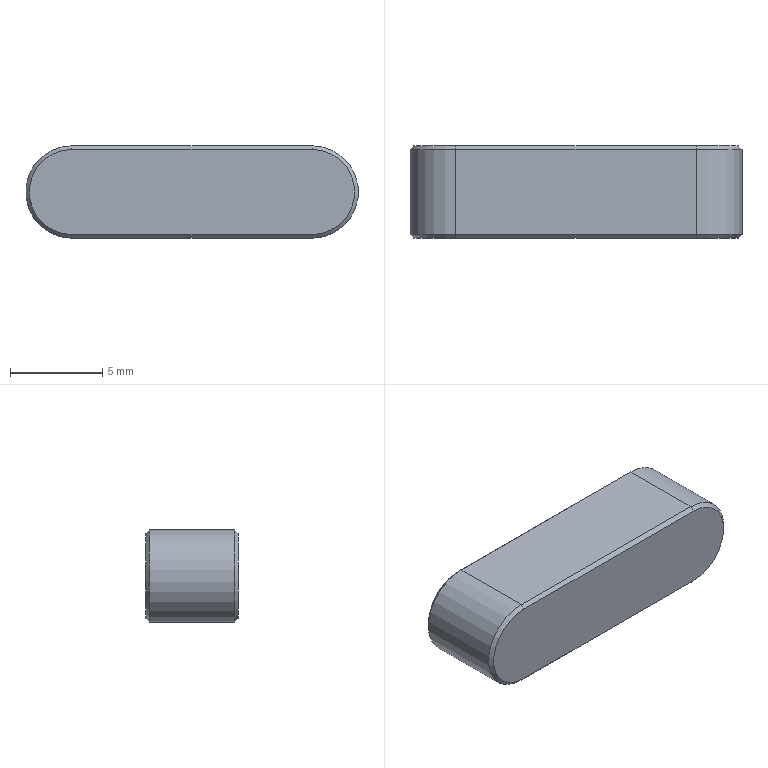Part | STEP file | KES5-18 | 1 solid | 14 faces | box 18 x 5 x 5 mm | volume 421.523 mm3 | plane 8 | cone 4 | cylinder 2 | commonest cylinder face diameters 5 x2
STEP:
#1=CARTESIAN_POINT('',(0.,0.,0.));
#2=DIRECTION('',(0.,0.,1.));
#3=DIRECTION('',(1.,0.,0.));
#4=AXIS2_PLACEMENT_3D('',#1,#2,#3);
#5=CARTESIAN_POINT('',(-6.5,4.8,-2.5));
#6=VERTEX_POINT('',#5);
#7=CARTESIAN_POINT('',(-6.5,0.2,-2.5));
#8=VERTEX_POINT('',#7);
#9=CARTESIAN_POINT('',(-6.5,5.,-2.5));
#10=DIRECTION('',(0.,-1.,0.));
#11=VECTOR('',#10,1.);
#12=LINE('',#9,#11);
#13=CARTESIAN_POINT('',(-6.5,5.,0.));
#14=DIRECTION('',(0.,-1.,0.));
#15=DIRECTION('',(0.,0.,-1.));
#16=AXIS2_PLACEMENT_3D('',#13,#14,#15);
#17=CYLINDRICAL_SURFACE('',#16,2.5);
#18=CARTESIAN_POINT('',(6.283,0.));
#19=DIRECTION('',(0.,1.));
#20=VECTOR('',#19,1.);
#21=LINE('',#18,#20);
#22=(GEOMETRIC_REPRESENTATION_CONTEXT(2)PARAMETRIC_REPRESENTATION_CONTEXT()REPRESENTATION_CONTEXT('',''));
#23=DEFINITIONAL_REPRESENTATION('',(#21),#22);
#24=PCURVE('',#17,#23);
#25=CARTESIAN_POINT('',(-14.672,5.,-2.5));
#26=DIRECTION('',(0.,0.,1.));
#27=DIRECTION('',(1.,0.,0.));
#28=AXIS2_PLACEMENT_3D('',#25,#26,#27);
#29=PLANE('',#28);
#30=CARTESIAN_POINT('',(8.172,0.));
#31=DIRECTION('',(0.,-1.));
#32=VECTOR('',#31,1.);
#33=LINE('',#30,#32);
#34=(GEOMETRIC_REPRESENTATION_CONTEXT(2)PARAMETRIC_REPRESENTATION_CONTEXT()REPRESENTATION_CONTEXT('',''));
#35=DEFINITIONAL_REPRESENTATION('',(#33),#34);
#36=PCURVE('',#29,#35);
#37=SURFACE_CURVE('',#12,(#24,#36),.PCURVE_S1.);
#38=EDGE_CURVE('',#6,#8,#37,.T.);
#39=ORIENTED_EDGE('',*,*,#38,.T.);
#40=CARTESIAN_POINT('',(-6.5,0.2,2.5));
#41=VERTEX_POINT('',#40);
#42=CARTESIAN_POINT('',(-6.5,0.2,0.));
#43=DIRECTION('',(0.,1.,0.));
#44=DIRECTION('',(0.,0.,1.));
#45=AXIS2_PLACEMENT_3D('',#42,#43,#44);
#46=CIRCLE('',#45,2.5);
#47=CARTESIAN_POINT('',(9.425,4.8));
#48=DIRECTION('',(-1.,0.));
#49=VECTOR('',#48,1.);
#50=LINE('',#47,#49);
#51=(GEOMETRIC_REPRESENTATION_CONTEXT(2)PARAMETRIC_REPRESENTATION_CONTEXT()REPRESENTATION_CONTEXT('',''));
#52=DEFINITIONAL_REPRESENTATION('',(#50),#51);
#53=PCURVE('',#17,#52);
#54=CARTESIAN_POINT('',(-6.5,0.2,0.));
#55=DIRECTION('',(0.,1.,0.));
#56=DIRECTION('',(0.,0.,1.));
#57=AXIS2_PLACEMENT_3D('',#54,#55,#56);
#58=CONICAL_SURFACE('',#57,2.5,0.7854);
#59=CARTESIAN_POINT('',(0.,0.));
#60=DIRECTION('',(1.,0.));
#61=VECTOR('',#60,1.);
#62=LINE('',#59,#61);
#63=(GEOMETRIC_REPRESENTATION_CONTEXT(2)PARAMETRIC_REPRESENTATION_CONTEXT()REPRESENTATION_CONTEXT('',''));
#64=DEFINITIONAL_REPRESENTATION('',(#62),#63);
#65=PCURVE('',#58,#64);
#66=SURFACE_CURVE('',#46,(#53,#65),.PCURVE_S1.);
#67=EDGE_CURVE('',#8,#41,#66,.T.);
#68=ORIENTED_EDGE('',*,*,#67,.T.);
#69=CARTESIAN_POINT('',(-6.5,4.8,2.5));
#70=VERTEX_POINT('',#69);
#71=CARTESIAN_POINT('',(-6.5,5.,2.5));
#72=DIRECTION('',(0.,-1.,0.));
#73=VECTOR('',#72,1.);
#74=LINE('',#71,#73);
#75=CARTESIAN_POINT('',(3.142,0.));
#76=DIRECTION('',(0.,1.));
#77=VECTOR('',#76,1.);
#78=LINE('',#75,#77);
#79=(GEOMETRIC_REPRESENTATION_CONTEXT(2)PARAMETRIC_REPRESENTATION_CONTEXT()REPRESENTATION_CONTEXT('',''));
#80=DEFINITIONAL_REPRESENTATION('',(#78),#79);
#81=PCURVE('',#17,#80);
#82=CARTESIAN_POINT('',(-14.672,5.,2.5));
#83=DIRECTION('',(0.,0.,1.));
#84=DIRECTION('',(1.,0.,0.));
#85=AXIS2_PLACEMENT_3D('',#82,#83,#84);
#86=PLANE('',#85);
#87=CARTESIAN_POINT('',(8.172,0.));
#88=DIRECTION('',(0.,-1.));
#89=VECTOR('',#88,1.);
#90=LINE('',#87,#89);
#91=(GEOMETRIC_REPRESENTATION_CONTEXT(2)PARAMETRIC_REPRESENTATION_CONTEXT()REPRESENTATION_CONTEXT('',''));
#92=DEFINITIONAL_REPRESENTATION('',(#90),#91);
#93=PCURVE('',#86,#92);
#94=SURFACE_CURVE('',#74,(#81,#93),.PCURVE_S1.);
#95=EDGE_CURVE('',#70,#41,#94,.T.);
#96=ORIENTED_EDGE('',*,*,#95,.F.);
#97=CARTESIAN_POINT('',(-6.5,4.8,0.));
#98=DIRECTION('',(0.,-1.,0.));
#99=DIRECTION('',(0.,0.,1.));
#100=AXIS2_PLACEMENT_3D('',#97,#98,#99);
#101=CIRCLE('',#100,2.5);
#102=CARTESIAN_POINT('',(3.142,0.2));
#103=DIRECTION('',(1.,0.));
#104=VECTOR('',#103,1.);
#105=LINE('',#102,#104);
#106=(GEOMETRIC_REPRESENTATION_CONTEXT(2)PARAMETRIC_REPRESENTATION_CONTEXT()REPRESENTATION_CONTEXT('',''));
#107=DEFINITIONAL_REPRESENTATION('',(#105),#106);
#108=PCURVE('',#17,#107);
#109=CARTESIAN_POINT('',(-6.5,5.,0.));
#110=DIRECTION('',(0.,-1.,0.));
#111=DIRECTION('',(0.,0.,-1.));
#112=AXIS2_PLACEMENT_3D('',#109,#110,#111);
#113=CONICAL_SURFACE('',#112,2.3,0.7854);
#114=CARTESIAN_POINT('',(3.142,0.2));
#115=DIRECTION('',(1.,0.));
#116=VECTOR('',#115,1.);
#117=LINE('',#114,#116);
#118=(GEOMETRIC_REPRESENTATION_CONTEXT(2)PARAMETRIC_REPRESENTATION_CONTEXT()REPRESENTATION_CONTEXT('',''));
#119=DEFINITIONAL_REPRESENTATION('',(#117),#118);
#120=PCURVE('',#113,#119);
#121=SURFACE_CURVE('',#101,(#108,#120),.PCURVE_S1.);
#122=EDGE_CURVE('',#70,#6,#121,.T.);
#123=ORIENTED_EDGE('',*,*,#122,.T.);
#124=EDGE_LOOP('',(#39,#68,#96,#123));
#125=FACE_BOUND('',#124,.T.);
#126=ADVANCED_FACE('',(#125),#17,.T.);
#127=ORIENTED_EDGE('',*,*,#95,.T.);
#128=CARTESIAN_POINT('',(6.5,0.2,2.5));
#129=VERTEX_POINT('',#128);
#130=CARTESIAN_POINT('',(6.5,0.2,2.5));
#131=DIRECTION('',(1.,0.,0.));
#132=VECTOR('',#131,1.);
#133=LINE('',#130,#132);
#134=CARTESIAN_POINT('',(21.172,-4.8));
#135=DIRECTION('',(1.,0.));
#136=VECTOR('',#135,1.);
#137=LINE('',#134,#136);
#138=(GEOMETRIC_REPRESENTATION_CONTEXT(2)PARAMETRIC_REPRESENTATION_CONTEXT()REPRESENTATION_CONTEXT('',''));
#139=DEFINITIONAL_REPRESENTATION('',(#137),#138);
#140=PCURVE('',#86,#139);
#141=CARTESIAN_POINT('',(-14.672,0.,2.3));
#142=DIRECTION('',(0.,-0.7071,0.7071));
#143=DIRECTION('',(0.,-0.7071,-0.7071));
#144=AXIS2_PLACEMENT_3D('',#141,#142,#143);
#145=PLANE('',#144);
#146=CARTESIAN_POINT('',(-0.2828,21.172));
#147=DIRECTION('',(0.,1.));
#148=VECTOR('',#147,1.);
#149=LINE('',#146,#148);
#150=(GEOMETRIC_REPRESENTATION_CONTEXT(2)PARAMETRIC_REPRESENTATION_CONTEXT()REPRESENTATION_CONTEXT('',''));
#151=DEFINITIONAL_REPRESENTATION('',(#149),#150);
#152=PCURVE('',#145,#151);
#153=SURFACE_CURVE('',#133,(#140,#152),.PCURVE_S1.);
#154=EDGE_CURVE('',#41,#129,#153,.T.);
#155=ORIENTED_EDGE('',*,*,#154,.T.);
#156=CARTESIAN_POINT('',(6.5,4.8,2.5));
#157=VERTEX_POINT('',#156);
#158=CARTESIAN_POINT('',(6.5,5.,2.5));
#159=DIRECTION('',(0.,-1.,0.));
#160=VECTOR('',#159,1.);
#161=LINE('',#158,#160);
#162=CARTESIAN_POINT('',(21.172,0.));
#163=DIRECTION('',(0.,-1.));
#164=VECTOR('',#163,1.);
#165=LINE('',#162,#164);
#166=(GEOMETRIC_REPRESENTATION_CONTEXT(2)PARAMETRIC_REPRESENTATION_CONTEXT()REPRESENTATION_CONTEXT('',''));
#167=DEFINITIONAL_REPRESENTATION('',(#165),#166);
#168=PCURVE('',#86,#167);
#169=CARTESIAN_POINT('',(6.5,5.,0.));
#170=DIRECTION('',(0.,-1.,0.));
#171=DIRECTION('',(0.,0.,-1.));
#172=AXIS2_PLACEMENT_3D('',#169,#170,#171);
#173=CYLINDRICAL_SURFACE('',#172,2.5);
#174=CARTESIAN_POINT('',(3.142,0.));
#175=DIRECTION('',(0.,1.));
#176=VECTOR('',#175,1.);
#177=LINE('',#174,#176);
#178=(GEOMETRIC_REPRESENTATION_CONTEXT(2)PARAMETRIC_REPRESENTATION_CONTEXT()REPRESENTATION_CONTEXT('',''));
#179=DEFINITIONAL_REPRESENTATION('',(#177),#178);
#180=PCURVE('',#173,#179);
#181=SURFACE_CURVE('',#161,(#168,#180),.PCURVE_S1.);
#182=EDGE_CURVE('',#157,#129,#181,.T.);
#183=ORIENTED_EDGE('',*,*,#182,.F.);
#184=CARTESIAN_POINT('',(-14.672,4.8,2.5));
#185=DIRECTION('',(-1.,0.,0.));
#186=VECTOR('',#185,1.);
#187=LINE('',#184,#186);
#188=CARTESIAN_POINT('',(0.,-0.2));
#189=DIRECTION('',(-1.,0.));
#190=VECTOR('',#189,1.);
#191=LINE('',#188,#190);
#192=(GEOMETRIC_REPRESENTATION_CONTEXT(2)PARAMETRIC_REPRESENTATION_CONTEXT()REPRESENTATION_CONTEXT('',''));
#193=DEFINITIONAL_REPRESENTATION('',(#191),#192);
#194=PCURVE('',#86,#193);
#195=CARTESIAN_POINT('',(-14.672,4.8,2.5));
#196=DIRECTION('',(0.,-0.7071,-0.7071));
#197=DIRECTION('',(0.,0.7071,-0.7071));
#198=AXIS2_PLACEMENT_3D('',#195,#196,#197);
#199=PLANE('',#198);
#200=CARTESIAN_POINT('',(0.,0.));
#201=DIRECTION('',(0.,-1.));
#202=VECTOR('',#201,1.);
#203=LINE('',#200,#202);
#204=(GEOMETRIC_REPRESENTATION_CONTEXT(2)PARAMETRIC_REPRESENTATION_CONTEXT()REPRESENTATION_CONTEXT('',''));
#205=DEFINITIONAL_REPRESENTATION('',(#203),#204);
#206=PCURVE('',#199,#205);
#207=SURFACE_CURVE('',#187,(#194,#206),.PCURVE_S1.);
#208=EDGE_CURVE('',#157,#70,#207,.T.);
#209=ORIENTED_EDGE('',*,*,#208,.T.);
#210=EDGE_LOOP('',(#127,#155,#183,#209));
#211=FACE_BOUND('',#210,.T.);
#212=ADVANCED_FACE('',(#211),#86,.T.);
#213=ORIENTED_EDGE('',*,*,#182,.T.);
#214=CARTESIAN_POINT('',(6.5,0.2,-2.5));
#215=VERTEX_POINT('',#214);
#216=CARTESIAN_POINT('',(6.5,0.2,0.));
#217=DIRECTION('',(0.,1.,0.));
#218=DIRECTION('',(0.,0.,1.));
#219=AXIS2_PLACEMENT_3D('',#216,#217,#218);
#220=CIRCLE('',#219,2.5);
#221=CARTESIAN_POINT('',(3.142,4.8));
#222=DIRECTION('',(-1.,0.));
#223=VECTOR('',#222,1.);
#224=LINE('',#221,#223);
#225=(GEOMETRIC_REPRESENTATION_CONTEXT(2)PARAMETRIC_REPRESENTATION_CONTEXT()REPRESENTATION_CONTEXT('',''));
#226=DEFINITIONAL_REPRESENTATION('',(#224),#225);
#227=PCURVE('',#173,#226);
#228=CARTESIAN_POINT('',(6.5,0.2,0.));
#229=DIRECTION('',(0.,1.,0.));
#230=DIRECTION('',(0.,0.,1.));
#231=AXIS2_PLACEMENT_3D('',#228,#229,#230);
#232=CONICAL_SURFACE('',#231,2.5,0.7854);
#233=CARTESIAN_POINT('',(0.,0.));
#234=DIRECTION('',(1.,0.));
#235=VECTOR('',#234,1.);
#236=LINE('',#233,#235);
#237=(GEOMETRIC_REPRESENTATION_CONTEXT(2)PARAMETRIC_REPRESENTATION_CONTEXT()REPRESENTATION_CONTEXT('',''));
#238=DEFINITIONAL_REPRESENTATION('',(#236),#237);
#239=PCURVE('',#232,#238);
#240=SURFACE_CURVE('',#220,(#227,#239),.PCURVE_S1.);
#241=EDGE_CURVE('',#129,#215,#240,.T.);
#242=ORIENTED_EDGE('',*,*,#241,.T.);
#243=CARTESIAN_POINT('',(6.5,4.8,-2.5));
#244=VERTEX_POINT('',#243);
#245=CARTESIAN_POINT('',(6.5,5.,-2.5));
#246=DIRECTION('',(0.,-1.,0.));
#247=VECTOR('',#246,1.);
#248=LINE('',#245,#247);
#249=CARTESIAN_POINT('',(0.,0.));
#250=DIRECTION('',(0.,1.));
#251=VECTOR('',#250,1.);
#252=LINE('',#249,#251);
#253=(GEOMETRIC_REPRESENTATION_CONTEXT(2)PARAMETRIC_REPRESENTATION_CONTEXT()REPRESENTATION_CONTEXT('',''));
#254=DEFINITIONAL_REPRESENTATION('',(#252),#253);
#255=PCURVE('',#173,#254);
#256=CARTESIAN_POINT('',(21.172,0.));
#257=DIRECTION('',(0.,-1.));
#258=VECTOR('',#257,1.);
#259=LINE('',#256,#258);
#260=(GEOMETRIC_REPRESENTATION_CONTEXT(2)PARAMETRIC_REPRESENTATION_CONTEXT()REPRESENTATION_CONTEXT('',''));
#261=DEFINITIONAL_REPRESENTATION('',(#259),#260);
#262=PCURVE('',#29,#261);
#263=SURFACE_CURVE('',#248,(#255,#262),.PCURVE_S1.);
#264=EDGE_CURVE('',#244,#215,#263,.T.);
#265=ORIENTED_EDGE('',*,*,#264,.F.);
#266=CARTESIAN_POINT('',(6.5,4.8,0.));
#267=DIRECTION('',(0.,-1.,0.));
#268=DIRECTION('',(0.,0.,1.));
#269=AXIS2_PLACEMENT_3D('',#266,#267,#268);
#270=CIRCLE('',#269,2.5);
#271=CARTESIAN_POINT('',(-3.142,0.2));
#272=DIRECTION('',(1.,0.));
#273=VECTOR('',#272,1.);
#274=LINE('',#271,#273);
#275=(GEOMETRIC_REPRESENTATION_CONTEXT(2)PARAMETRIC_REPRESENTATION_CONTEXT()REPRESENTATION_CONTEXT('',''));
#276=DEFINITIONAL_REPRESENTATION('',(#274),#275);
#277=PCURVE('',#173,#276);
#278=CARTESIAN_POINT('',(6.5,5.,0.));
#279=DIRECTION('',(0.,-1.,0.));
#280=DIRECTION('',(0.,0.,-1.));
#281=AXIS2_PLACEMENT_3D('',#278,#279,#280);
#282=CONICAL_SURFACE('',#281,2.3,0.7854);
#283=CARTESIAN_POINT('',(-3.142,0.2));
#284=DIRECTION('',(1.,0.));
#285=VECTOR('',#284,1.);
#286=LINE('',#283,#285);
#287=(GEOMETRIC_REPRESENTATION_CONTEXT(2)PARAMETRIC_REPRESENTATION_CONTEXT()REPRESENTATION_CONTEXT('',''));
#288=DEFINITIONAL_REPRESENTATION('',(#286),#287);
#289=PCURVE('',#282,#288);
#290=SURFACE_CURVE('',#270,(#277,#289),.PCURVE_S1.);
#291=EDGE_CURVE('',#244,#157,#290,.T.);
#292=ORIENTED_EDGE('',*,*,#291,.T.);
#293=EDGE_LOOP('',(#213,#242,#265,#292));
#294=FACE_BOUND('',#293,.T.);
#295=ADVANCED_FACE('',(#294),#173,.T.);
#296=ORIENTED_EDGE('',*,*,#264,.T.);
#297=CARTESIAN_POINT('',(-14.672,0.2,-2.5));
#298=DIRECTION('',(-1.,0.,0.));
#299=VECTOR('',#298,1.);
#300=LINE('',#297,#299);
#301=CARTESIAN_POINT('',(0.,-4.8));
#302=DIRECTION('',(-1.,0.));
#303=VECTOR('',#302,1.);
#304=LINE('',#301,#303);
#305=(GEOMETRIC_REPRESENTATION_CONTEXT(2)PARAMETRIC_REPRESENTATION_CONTEXT()REPRESENTATION_CONTEXT('',''));
#306=DEFINITIONAL_REPRESENTATION('',(#304),#305);
#307=PCURVE('',#29,#306);
#308=CARTESIAN_POINT('',(-14.672,0.2,-2.5));
#309=DIRECTION('',(0.,0.7071,0.7071));
#310=DIRECTION('',(0.,-0.7071,0.7071));
#311=AXIS2_PLACEMENT_3D('',#308,#309,#310);
#312=PLANE('',#311);
#313=CARTESIAN_POINT('',(0.,0.));
#314=DIRECTION('',(0.,-1.));
#315=VECTOR('',#314,1.);
#316=LINE('',#313,#315);
#317=(GEOMETRIC_REPRESENTATION_CONTEXT(2)PARAMETRIC_REPRESENTATION_CONTEXT()REPRESENTATION_CONTEXT('',''));
#318=DEFINITIONAL_REPRESENTATION('',(#316),#317);
#319=PCURVE('',#312,#318);
#320=SURFACE_CURVE('',#300,(#307,#319),.PCURVE_S1.);
#321=EDGE_CURVE('',#215,#8,#320,.T.);
#322=ORIENTED_EDGE('',*,*,#321,.T.);
#323=ORIENTED_EDGE('',*,*,#38,.F.);
#324=CARTESIAN_POINT('',(6.5,4.8,-2.5));
#325=DIRECTION('',(1.,0.,0.));
#326=VECTOR('',#325,1.);
#327=LINE('',#324,#326);
#328=CARTESIAN_POINT('',(21.172,-0.2));
#329=DIRECTION('',(1.,0.));
#330=VECTOR('',#329,1.);
#331=LINE('',#328,#330);
#332=(GEOMETRIC_REPRESENTATION_CONTEXT(2)PARAMETRIC_REPRESENTATION_CONTEXT()REPRESENTATION_CONTEXT('',''));
#333=DEFINITIONAL_REPRESENTATION('',(#331),#332);
#334=PCURVE('',#29,#333);
#335=CARTESIAN_POINT('',(-14.672,5.,-2.3));
#336=DIRECTION('',(0.,0.7071,-0.7071));
#337=DIRECTION('',(0.,0.7071,0.7071));
#338=AXIS2_PLACEMENT_3D('',#335,#336,#337);
#339=PLANE('',#338);
#340=CARTESIAN_POINT('',(-0.2828,21.172));
#341=DIRECTION('',(0.,1.));
#342=VECTOR('',#341,1.);
#343=LINE('',#340,#342);
#344=(GEOMETRIC_REPRESENTATION_CONTEXT(2)PARAMETRIC_REPRESENTATION_CONTEXT()REPRESENTATION_CONTEXT('',''));
#345=DEFINITIONAL_REPRESENTATION('',(#343),#344);
#346=PCURVE('',#339,#345);
#347=SURFACE_CURVE('',#327,(#334,#346),.PCURVE_S1.);
#348=EDGE_CURVE('',#6,#244,#347,.T.);
#349=ORIENTED_EDGE('',*,*,#348,.T.);
#350=EDGE_LOOP('',(#296,#322,#323,#349));
#351=FACE_BOUND('',#350,.T.);
#352=ADVANCED_FACE('',(#351),#29,.F.);
#353=CARTESIAN_POINT('',(-6.5,5.,2.3));
#354=VERTEX_POINT('',#353);
#355=CARTESIAN_POINT('',(6.5,5.,2.3));
#356=VERTEX_POINT('',#355);
#357=CARTESIAN_POINT('',(-14.672,5.,2.3));
#358=DIRECTION('',(1.,0.,0.));
#359=VECTOR('',#358,1.);
#360=LINE('',#357,#359);
#361=CARTESIAN_POINT('',(-14.672,5.,0.));
#362=DIRECTION('',(0.,1.,0.));
#363=DIRECTION('',(0.,0.,1.));
#364=AXIS2_PLACEMENT_3D('',#361,#362,#363);
#365=PLANE('',#364);
#366=CARTESIAN_POINT('',(2.3,0.));
#367=DIRECTION('',(0.,1.));
#368=VECTOR('',#367,1.);
#369=LINE('',#366,#368);
#370=(GEOMETRIC_REPRESENTATION_CONTEXT(2)PARAMETRIC_REPRESENTATION_CONTEXT()REPRESENTATION_CONTEXT('',''));
#371=DEFINITIONAL_REPRESENTATION('',(#369),#370);
#372=PCURVE('',#365,#371);
#373=CARTESIAN_POINT('',(0.2828,0.));
#374=DIRECTION('',(0.,1.));
#375=VECTOR('',#374,1.);
#376=LINE('',#373,#375);
#377=(GEOMETRIC_REPRESENTATION_CONTEXT(2)PARAMETRIC_REPRESENTATION_CONTEXT()REPRESENTATION_CONTEXT('',''));
#378=DEFINITIONAL_REPRESENTATION('',(#376),#377);
#379=PCURVE('',#199,#378);
#380=SURFACE_CURVE('',#360,(#372,#379),.PCURVE_S1.);
#381=EDGE_CURVE('',#354,#356,#380,.T.);
#382=ORIENTED_EDGE('',*,*,#381,.T.);
#383=CARTESIAN_POINT('',(6.5,5.,-2.3));
#384=VERTEX_POINT('',#383);
#385=CARTESIAN_POINT('',(6.5,5.,0.));
#386=DIRECTION('',(0.,1.,0.));
#387=DIRECTION('',(0.,0.,1.));
#388=AXIS2_PLACEMENT_3D('',#385,#386,#387);
#389=CIRCLE('',#388,2.3);
#390=CARTESIAN_POINT('',(0.,21.172));
#391=DIRECTION('',(1.,0.));
#392=AXIS2_PLACEMENT_2D('',#390,#391);
#393=CIRCLE('',#392,2.3);
#394=(GEOMETRIC_REPRESENTATION_CONTEXT(2)PARAMETRIC_REPRESENTATION_CONTEXT()REPRESENTATION_CONTEXT('',''));
#395=DEFINITIONAL_REPRESENTATION('',(#393),#394);
#396=PCURVE('',#365,#395);
#397=CARTESIAN_POINT('',(3.142,0.));
#398=DIRECTION('',(-1.,0.));
#399=VECTOR('',#398,1.);
#400=LINE('',#397,#399);
#401=(GEOMETRIC_REPRESENTATION_CONTEXT(2)PARAMETRIC_REPRESENTATION_CONTEXT()REPRESENTATION_CONTEXT('',''));
#402=DEFINITIONAL_REPRESENTATION('',(#400),#401);
#403=PCURVE('',#282,#402);
#404=SURFACE_CURVE('',#389,(#396,#403),.PCURVE_S1.);
#405=EDGE_CURVE('',#356,#384,#404,.T.);
#406=ORIENTED_EDGE('',*,*,#405,.T.);
#407=CARTESIAN_POINT('',(-6.5,5.,-2.3));
#408=VERTEX_POINT('',#407);
#409=CARTESIAN_POINT('',(-6.5,5.,-2.3));
#410=DIRECTION('',(-1.,0.,0.));
#411=VECTOR('',#410,1.);
#412=LINE('',#409,#411);
#413=CARTESIAN_POINT('',(-2.3,8.172));
#414=DIRECTION('',(0.,-1.));
#415=VECTOR('',#414,1.);
#416=LINE('',#413,#415);
#417=(GEOMETRIC_REPRESENTATION_CONTEXT(2)PARAMETRIC_REPRESENTATION_CONTEXT()REPRESENTATION_CONTEXT('',''));
#418=DEFINITIONAL_REPRESENTATION('',(#416),#417);
#419=PCURVE('',#365,#418);
#420=CARTESIAN_POINT('',(0.,8.172));
#421=DIRECTION('',(0.,-1.));
#422=VECTOR('',#421,1.);
#423=LINE('',#420,#422);
#424=(GEOMETRIC_REPRESENTATION_CONTEXT(2)PARAMETRIC_REPRESENTATION_CONTEXT()REPRESENTATION_CONTEXT('',''));
#425=DEFINITIONAL_REPRESENTATION('',(#423),#424);
#426=PCURVE('',#339,#425);
#427=SURFACE_CURVE('',#412,(#419,#426),.PCURVE_S1.);
#428=EDGE_CURVE('',#384,#408,#427,.T.);
#429=ORIENTED_EDGE('',*,*,#428,.T.);
#430=CARTESIAN_POINT('',(-6.5,5.,0.));
#431=DIRECTION('',(0.,1.,0.));
#432=DIRECTION('',(0.,0.,1.));
#433=AXIS2_PLACEMENT_3D('',#430,#431,#432);
#434=CIRCLE('',#433,2.3);
#435=CARTESIAN_POINT('',(0.,8.172));
#436=DIRECTION('',(1.,0.));
#437=AXIS2_PLACEMENT_2D('',#435,#436);
#438=CIRCLE('',#437,2.3);
#439=(GEOMETRIC_REPRESENTATION_CONTEXT(2)PARAMETRIC_REPRESENTATION_CONTEXT()REPRESENTATION_CONTEXT('',''));
#440=DEFINITIONAL_REPRESENTATION('',(#438),#439);
#441=PCURVE('',#365,#440);
#442=CARTESIAN_POINT('',(9.425,0.));
#443=DIRECTION('',(-1.,0.));
#444=VECTOR('',#443,1.);
#445=LINE('',#442,#444);
#446=(GEOMETRIC_REPRESENTATION_CONTEXT(2)PARAMETRIC_REPRESENTATION_CONTEXT()REPRESENTATION_CONTEXT('',''));
#447=DEFINITIONAL_REPRESENTATION('',(#445),#446);
#448=PCURVE('',#113,#447);
#449=SURFACE_CURVE('',#434,(#441,#448),.PCURVE_S1.);
#450=EDGE_CURVE('',#408,#354,#449,.T.);
#451=ORIENTED_EDGE('',*,*,#450,.T.);
#452=EDGE_LOOP('',(#382,#406,#429,#451));
#453=FACE_BOUND('',#452,.T.);
#454=ADVANCED_FACE('',(#453),#365,.T.);
#455=CARTESIAN_POINT('',(-6.5,0.,2.3));
#456=VERTEX_POINT('',#455);
#457=CARTESIAN_POINT('',(-6.5,0.,-2.3));
#458=VERTEX_POINT('',#457);
#459=CARTESIAN_POINT('',(-6.5,0.,0.));
#460=DIRECTION('',(0.,-1.,0.));
#461=DIRECTION('',(0.,0.,1.));
#462=AXIS2_PLACEMENT_3D('',#459,#460,#461);
#463=CIRCLE('',#462,2.3);
#464=CARTESIAN_POINT('',(-14.672,0.,0.));
#465=DIRECTION('',(0.,1.,0.));
#466=DIRECTION('',(0.,0.,1.));
#467=AXIS2_PLACEMENT_3D('',#464,#465,#466);
#468=PLANE('',#467);
#469=CARTESIAN_POINT('',(2.3,8.172));
#470=CARTESIAN_POINT('',(2.3,4.189));
#471=CARTESIAN_POINT('',(-1.15,6.18));
#472=CARTESIAN_POINT('',(-4.6,8.172));
#473=CARTESIAN_POINT('',(-1.15,10.164));
#474=CARTESIAN_POINT('',(2.3,12.156));
#475=CARTESIAN_POINT('',(2.3,8.172));
#476=(BOUNDED_CURVE()B_SPLINE_CURVE(2,(#469,#470,#471,#472,#473,#474,#475),.UNSPECIFIED.,.T.,.F.)B_SPLINE_CURVE_WITH_KNOTS((1,2,2,2,2,1),(-2.094,0.,2.094,4.189,6.283,8.378),.UNSPECIFIED.)CURVE()GEOMETRIC_REPRESENTATION_ITEM()RATIONAL_B_SPLINE_CURVE((1.,0.5,1.,0.5,1.,0.5,1.))REPRESENTATION_ITEM(''));
#477=(GEOMETRIC_REPRESENTATION_CONTEXT(2)PARAMETRIC_REPRESENTATION_CONTEXT()REPRESENTATION_CONTEXT('',''));
#478=DEFINITIONAL_REPRESENTATION('',(#476),#477);
#479=PCURVE('',#468,#478);
#480=CARTESIAN_POINT('',(6.283,-0.2));
#481=DIRECTION('',(-1.,0.));
#482=VECTOR('',#481,1.);
#483=LINE('',#480,#482);
#484=(GEOMETRIC_REPRESENTATION_CONTEXT(2)PARAMETRIC_REPRESENTATION_CONTEXT()REPRESENTATION_CONTEXT('',''));
#485=DEFINITIONAL_REPRESENTATION('',(#483),#484);
#486=PCURVE('',#58,#485);
#487=SURFACE_CURVE('',#463,(#479,#486),.PCURVE_S1.);
#488=EDGE_CURVE('',#456,#458,#487,.T.);
#489=ORIENTED_EDGE('',*,*,#488,.T.);
#490=CARTESIAN_POINT('',(6.5,0.,-2.3));
#491=VERTEX_POINT('',#490);
#492=CARTESIAN_POINT('',(-14.672,0.,-2.3));
#493=DIRECTION('',(1.,0.,0.));
#494=VECTOR('',#493,1.);
#495=LINE('',#492,#494);
#496=CARTESIAN_POINT('',(-2.3,0.));
#497=DIRECTION('',(0.,1.));
#498=VECTOR('',#497,1.);
#499=LINE('',#496,#498);
#500=(GEOMETRIC_REPRESENTATION_CONTEXT(2)PARAMETRIC_REPRESENTATION_CONTEXT()REPRESENTATION_CONTEXT('',''));
#501=DEFINITIONAL_REPRESENTATION('',(#499),#500);
#502=PCURVE('',#468,#501);
#503=CARTESIAN_POINT('',(0.2828,0.));
#504=DIRECTION('',(0.,1.));
#505=VECTOR('',#504,1.);
#506=LINE('',#503,#505);
#507=(GEOMETRIC_REPRESENTATION_CONTEXT(2)PARAMETRIC_REPRESENTATION_CONTEXT()REPRESENTATION_CONTEXT('',''));
#508=DEFINITIONAL_REPRESENTATION('',(#506),#507);
#509=PCURVE('',#312,#508);
#510=SURFACE_CURVE('',#495,(#502,#509),.PCURVE_S1.);
#511=EDGE_CURVE('',#458,#491,#510,.T.);
#512=ORIENTED_EDGE('',*,*,#511,.T.);
#513=CARTESIAN_POINT('',(6.5,0.,2.3));
#514=VERTEX_POINT('',#513);
#515=CARTESIAN_POINT('',(6.5,0.,0.));
#516=DIRECTION('',(0.,-1.,0.));
#517=DIRECTION('',(0.,0.,1.));
#518=AXIS2_PLACEMENT_3D('',#515,#516,#517);
#519=CIRCLE('',#518,2.3);
#520=CARTESIAN_POINT('',(2.3,21.172));
#521=CARTESIAN_POINT('',(2.3,17.189));
#522=CARTESIAN_POINT('',(-1.15,19.18));
#523=CARTESIAN_POINT('',(-4.6,21.172));
#524=CARTESIAN_POINT('',(-1.15,23.164));
#525=CARTESIAN_POINT('',(2.3,25.156));
#526=CARTESIAN_POINT('',(2.3,21.172));
#527=(BOUNDED_CURVE()B_SPLINE_CURVE(2,(#520,#521,#522,#523,#524,#525,#526),.UNSPECIFIED.,.T.,.F.)B_SPLINE_CURVE_WITH_KNOTS((1,2,2,2,2,1),(-2.094,0.,2.094,4.189,6.283,8.378),.UNSPECIFIED.)CURVE()GEOMETRIC_REPRESENTATION_ITEM()RATIONAL_B_SPLINE_CURVE((1.,0.5,1.,0.5,1.,0.5,1.))REPRESENTATION_ITEM(''));
#528=(GEOMETRIC_REPRESENTATION_CONTEXT(2)PARAMETRIC_REPRESENTATION_CONTEXT()REPRESENTATION_CONTEXT('',''));
#529=DEFINITIONAL_REPRESENTATION('',(#527),#528);
#530=PCURVE('',#468,#529);
#531=CARTESIAN_POINT('',(6.283,-0.2));
#532=DIRECTION('',(-1.,0.));
#533=VECTOR('',#532,1.);
#534=LINE('',#531,#533);
#535=(GEOMETRIC_REPRESENTATION_CONTEXT(2)PARAMETRIC_REPRESENTATION_CONTEXT()REPRESENTATION_CONTEXT('',''));
#536=DEFINITIONAL_REPRESENTATION('',(#534),#535);
#537=PCURVE('',#232,#536);
#538=SURFACE_CURVE('',#519,(#530,#537),.PCURVE_S1.);
#539=EDGE_CURVE('',#491,#514,#538,.T.);
#540=ORIENTED_EDGE('',*,*,#539,.T.);
#541=CARTESIAN_POINT('',(-6.5,0.,2.3));
#542=DIRECTION('',(-1.,0.,0.));
#543=VECTOR('',#542,1.);
#544=LINE('',#541,#543);
#545=CARTESIAN_POINT('',(2.3,8.172));
#546=DIRECTION('',(0.,-1.));
#547=VECTOR('',#546,1.);
#548=LINE('',#545,#547);
#549=(GEOMETRIC_REPRESENTATION_CONTEXT(2)PARAMETRIC_REPRESENTATION_CONTEXT()REPRESENTATION_CONTEXT('',''));
#550=DEFINITIONAL_REPRESENTATION('',(#548),#549);
#551=PCURVE('',#468,#550);
#552=CARTESIAN_POINT('',(0.,8.172));
#553=DIRECTION('',(0.,-1.));
#554=VECTOR('',#553,1.);
#555=LINE('',#552,#554);
#556=(GEOMETRIC_REPRESENTATION_CONTEXT(2)PARAMETRIC_REPRESENTATION_CONTEXT()REPRESENTATION_CONTEXT('',''));
#557=DEFINITIONAL_REPRESENTATION('',(#555),#556);
#558=PCURVE('',#145,#557);
#559=SURFACE_CURVE('',#544,(#551,#558),.PCURVE_S1.);
#560=EDGE_CURVE('',#514,#456,#559,.T.);
#561=ORIENTED_EDGE('',*,*,#560,.T.);
#562=EDGE_LOOP('',(#489,#512,#540,#561));
#563=FACE_BOUND('',#562,.T.);
#564=ADVANCED_FACE('',(#563),#468,.F.);
#565=CARTESIAN_POINT('',(-6.5,0.,2.3));
#566=DIRECTION('',(0.,0.7071,0.7071));
#567=VECTOR('',#566,1.);
#568=LINE('',#565,#567);
#569=CARTESIAN_POINT('',(0.,8.172));
#570=DIRECTION('',(-1.,0.));
#571=VECTOR('',#570,1.);
#572=LINE('',#569,#571);
#573=(GEOMETRIC_REPRESENTATION_CONTEXT(2)PARAMETRIC_REPRESENTATION_CONTEXT()REPRESENTATION_CONTEXT('',''));
#574=DEFINITIONAL_REPRESENTATION('',(#572),#573);
#575=PCURVE('',#145,#574);
#576=CARTESIAN_POINT('',(6.283,-0.2));
#577=DIRECTION('',(0.,1.));
#578=VECTOR('',#577,1.);
#579=LINE('',#576,#578);
#580=(GEOMETRIC_REPRESENTATION_CONTEXT(2)PARAMETRIC_REPRESENTATION_CONTEXT()REPRESENTATION_CONTEXT('',''));
#581=DEFINITIONAL_REPRESENTATION('',(#579),#580);
#582=PCURVE('',#58,#581);
#583=SURFACE_CURVE('',#568,(#575,#582),.PCURVE_S1.);
#584=EDGE_CURVE('',#456,#41,#583,.T.);
#585=ORIENTED_EDGE('',*,*,#584,.F.);
#586=ORIENTED_EDGE('',*,*,#560,.F.);
#587=CARTESIAN_POINT('',(6.5,0.2,2.5));
#588=DIRECTION('',(0.,-0.7071,-0.7071));
#589=VECTOR('',#588,1.);
#590=LINE('',#587,#589);
#591=CARTESIAN_POINT('',(-0.2828,21.172));
#592=DIRECTION('',(1.,0.));
#593=VECTOR('',#592,1.);
#594=LINE('',#591,#593);
#595=(GEOMETRIC_REPRESENTATION_CONTEXT(2)PARAMETRIC_REPRESENTATION_CONTEXT()REPRESENTATION_CONTEXT('',''));
#596=DEFINITIONAL_REPRESENTATION('',(#594),#595);
#597=PCURVE('',#145,#596);
#598=CARTESIAN_POINT('',(0.,0.));
#599=DIRECTION('',(0.,-1.));
#600=VECTOR('',#599,1.);
#601=LINE('',#598,#600);
#602=(GEOMETRIC_REPRESENTATION_CONTEXT(2)PARAMETRIC_REPRESENTATION_CONTEXT()REPRESENTATION_CONTEXT('',''));
#603=DEFINITIONAL_REPRESENTATION('',(#601),#602);
#604=PCURVE('',#232,#603);
#605=SURFACE_CURVE('',#590,(#597,#604),.PCURVE_S1.);
#606=EDGE_CURVE('',#129,#514,#605,.T.);
#607=ORIENTED_EDGE('',*,*,#606,.F.);
#608=ORIENTED_EDGE('',*,*,#154,.F.);
#609=EDGE_LOOP('',(#585,#586,#607,#608));
#610=FACE_BOUND('',#609,.T.);
#611=ADVANCED_FACE('',(#610),#145,.T.);
#612=ORIENTED_EDGE('',*,*,#606,.T.);
#613=ORIENTED_EDGE('',*,*,#539,.F.);
#614=CARTESIAN_POINT('',(6.5,0.2,-2.5));
#615=DIRECTION('',(0.,-0.7071,0.7071));
#616=VECTOR('',#615,1.);
#617=LINE('',#614,#616);
#618=CARTESIAN_POINT('',(3.142,0.));
#619=DIRECTION('',(0.,-1.));
#620=VECTOR('',#619,1.);
#621=LINE('',#618,#620);
#622=(GEOMETRIC_REPRESENTATION_CONTEXT(2)PARAMETRIC_REPRESENTATION_CONTEXT()REPRESENTATION_CONTEXT('',''));
#623=DEFINITIONAL_REPRESENTATION('',(#621),#622);
#624=PCURVE('',#232,#623);
#625=CARTESIAN_POINT('',(0.,21.172));
#626=DIRECTION('',(1.,0.));
#627=VECTOR('',#626,1.);
#628=LINE('',#625,#627);
#629=(GEOMETRIC_REPRESENTATION_CONTEXT(2)PARAMETRIC_REPRESENTATION_CONTEXT()REPRESENTATION_CONTEXT('',''));
#630=DEFINITIONAL_REPRESENTATION('',(#628),#629);
#631=PCURVE('',#312,#630);
#632=SURFACE_CURVE('',#617,(#624,#631),.PCURVE_S1.);
#633=EDGE_CURVE('',#215,#491,#632,.T.);
#634=ORIENTED_EDGE('',*,*,#633,.F.);
#635=ORIENTED_EDGE('',*,*,#241,.F.);
#636=EDGE_LOOP('',(#612,#613,#634,#635));
#637=FACE_BOUND('',#636,.T.);
#638=ADVANCED_FACE('',(#637),#232,.T.);
#639=ORIENTED_EDGE('',*,*,#584,.T.);
#640=ORIENTED_EDGE('',*,*,#67,.F.);
#641=CARTESIAN_POINT('',(-6.5,0.,-2.3));
#642=DIRECTION('',(0.,0.7071,-0.7071));
#643=VECTOR('',#642,1.);
#644=LINE('',#641,#643);
#645=CARTESIAN_POINT('',(3.142,-0.2));
#646=DIRECTION('',(0.,1.));
#647=VECTOR('',#646,1.);
#648=LINE('',#645,#647);
#649=(GEOMETRIC_REPRESENTATION_CONTEXT(2)PARAMETRIC_REPRESENTATION_CONTEXT()REPRESENTATION_CONTEXT('',''));
#650=DEFINITIONAL_REPRESENTATION('',(#648),#649);
#651=PCURVE('',#58,#650);
#652=CARTESIAN_POINT('',(0.2828,8.172));
#653=DIRECTION('',(-1.,0.));
#654=VECTOR('',#653,1.);
#655=LINE('',#652,#654);
#656=(GEOMETRIC_REPRESENTATION_CONTEXT(2)PARAMETRIC_REPRESENTATION_CONTEXT()REPRESENTATION_CONTEXT('',''));
#657=DEFINITIONAL_REPRESENTATION('',(#655),#656);
#658=PCURVE('',#312,#657);
#659=SURFACE_CURVE('',#644,(#651,#658),.PCURVE_S1.);
#660=EDGE_CURVE('',#458,#8,#659,.T.);
#661=ORIENTED_EDGE('',*,*,#660,.F.);
#662=ORIENTED_EDGE('',*,*,#488,.F.);
#663=EDGE_LOOP('',(#639,#640,#661,#662));
#664=FACE_BOUND('',#663,.T.);
#665=ADVANCED_FACE('',(#664),#58,.T.);
#666=ORIENTED_EDGE('',*,*,#633,.T.);
#667=ORIENTED_EDGE('',*,*,#511,.F.);
#668=ORIENTED_EDGE('',*,*,#660,.T.);
#669=ORIENTED_EDGE('',*,*,#321,.F.);
#670=EDGE_LOOP('',(#666,#667,#668,#669));
#671=FACE_BOUND('',#670,.T.);
#672=ADVANCED_FACE('',(#671),#312,.F.);
#673=CARTESIAN_POINT('',(-6.5,4.8,-2.5));
#674=DIRECTION('',(0.,0.7071,0.7071));
#675=VECTOR('',#674,1.);
#676=LINE('',#673,#675);
#677=CARTESIAN_POINT('',(6.283,0.2));
#678=DIRECTION('',(0.,-1.));
#679=VECTOR('',#678,1.);
#680=LINE('',#677,#679);
#681=(GEOMETRIC_REPRESENTATION_CONTEXT(2)PARAMETRIC_REPRESENTATION_CONTEXT()REPRESENTATION_CONTEXT('',''));
#682=DEFINITIONAL_REPRESENTATION('',(#680),#681);
#683=PCURVE('',#113,#682);
#684=CARTESIAN_POINT('',(-0.2828,8.172));
#685=DIRECTION('',(1.,0.));
#686=VECTOR('',#685,1.);
#687=LINE('',#684,#686);
#688=(GEOMETRIC_REPRESENTATION_CONTEXT(2)PARAMETRIC_REPRESENTATION_CONTEXT()REPRESENTATION_CONTEXT('',''));
#689=DEFINITIONAL_REPRESENTATION('',(#687),#688);
#690=PCURVE('',#339,#689);
#691=SURFACE_CURVE('',#676,(#683,#690),.PCURVE_S1.);
#692=EDGE_CURVE('',#6,#408,#691,.T.);
#693=ORIENTED_EDGE('',*,*,#692,.F.);
#694=ORIENTED_EDGE('',*,*,#122,.F.);
#695=CARTESIAN_POINT('',(-6.5,5.,2.3));
#696=DIRECTION('',(0.,-0.7071,0.7071));
#697=VECTOR('',#696,1.);
#698=LINE('',#695,#697);
#699=CARTESIAN_POINT('',(3.142,0.));
#700=DIRECTION('',(0.,1.));
#701=VECTOR('',#700,1.);
#702=LINE('',#699,#701);
#703=(GEOMETRIC_REPRESENTATION_CONTEXT(2)PARAMETRIC_REPRESENTATION_CONTEXT()REPRESENTATION_CONTEXT('',''));
#704=DEFINITIONAL_REPRESENTATION('',(#702),#703);
#705=PCURVE('',#113,#704);
#706=CARTESIAN_POINT('',(0.2828,8.172));
#707=DIRECTION('',(-1.,0.));
#708=VECTOR('',#707,1.);
#709=LINE('',#706,#708);
#710=(GEOMETRIC_REPRESENTATION_CONTEXT(2)PARAMETRIC_REPRESENTATION_CONTEXT()REPRESENTATION_CONTEXT('',''));
#711=DEFINITIONAL_REPRESENTATION('',(#709),#710);
#712=PCURVE('',#199,#711);
#713=SURFACE_CURVE('',#698,(#705,#712),.PCURVE_S1.);
#714=EDGE_CURVE('',#354,#70,#713,.T.);
#715=ORIENTED_EDGE('',*,*,#714,.F.);
#716=ORIENTED_EDGE('',*,*,#450,.F.);
#717=EDGE_LOOP('',(#693,#694,#715,#716));
#718=FACE_BOUND('',#717,.T.);
#719=ADVANCED_FACE('',(#718),#113,.T.);
#720=ORIENTED_EDGE('',*,*,#714,.T.);
#721=ORIENTED_EDGE('',*,*,#208,.F.);
#722=CARTESIAN_POINT('',(6.5,5.,2.3));
#723=DIRECTION('',(0.,-0.7071,0.7071));
#724=VECTOR('',#723,1.);
#725=LINE('',#722,#724);
#726=CARTESIAN_POINT('',(0.2828,21.172));
#727=DIRECTION('',(-1.,0.));
#728=VECTOR('',#727,1.);
#729=LINE('',#726,#728);
#730=(GEOMETRIC_REPRESENTATION_CONTEXT(2)PARAMETRIC_REPRESENTATION_CONTEXT()REPRESENTATION_CONTEXT('',''));
#731=DEFINITIONAL_REPRESENTATION('',(#729),#730);
#732=PCURVE('',#199,#731);
#733=CARTESIAN_POINT('',(3.142,0.));
#734=DIRECTION('',(0.,1.));
#735=VECTOR('',#734,1.);
#736=LINE('',#733,#735);
#737=(GEOMETRIC_REPRESENTATION_CONTEXT(2)PARAMETRIC_REPRESENTATION_CONTEXT()REPRESENTATION_CONTEXT('',''));
#738=DEFINITIONAL_REPRESENTATION('',(#736),#737);
#739=PCURVE('',#282,#738);
#740=SURFACE_CURVE('',#725,(#732,#739),.PCURVE_S1.);
#741=EDGE_CURVE('',#356,#157,#740,.T.);
#742=ORIENTED_EDGE('',*,*,#741,.F.);
#743=ORIENTED_EDGE('',*,*,#381,.F.);
#744=EDGE_LOOP('',(#720,#721,#742,#743));
#745=FACE_BOUND('',#744,.T.);
#746=ADVANCED_FACE('',(#745),#199,.F.);
#747=ORIENTED_EDGE('',*,*,#692,.T.);
#748=ORIENTED_EDGE('',*,*,#428,.F.);
#749=CARTESIAN_POINT('',(6.5,4.8,-2.5));
#750=DIRECTION('',(0.,0.7071,0.7071));
#751=VECTOR('',#750,1.);
#752=LINE('',#749,#751);
#753=CARTESIAN_POINT('',(-0.2828,21.172));
#754=DIRECTION('',(1.,0.));
#755=VECTOR('',#754,1.);
#756=LINE('',#753,#755);
#757=(GEOMETRIC_REPRESENTATION_CONTEXT(2)PARAMETRIC_REPRESENTATION_CONTEXT()REPRESENTATION_CONTEXT('',''));
#758=DEFINITIONAL_REPRESENTATION('',(#756),#757);
#759=PCURVE('',#339,#758);
#760=CARTESIAN_POINT('',(0.,0.2));
#761=DIRECTION('',(0.,-1.));
#762=VECTOR('',#761,1.);
#763=LINE('',#760,#762);
#764=(GEOMETRIC_REPRESENTATION_CONTEXT(2)PARAMETRIC_REPRESENTATION_CONTEXT()REPRESENTATION_CONTEXT('',''));
#765=DEFINITIONAL_REPRESENTATION('',(#763),#764);
#766=PCURVE('',#282,#765);
#767=SURFACE_CURVE('',#752,(#759,#766),.PCURVE_S1.);
#768=EDGE_CURVE('',#244,#384,#767,.T.);
#769=ORIENTED_EDGE('',*,*,#768,.F.);
#770=ORIENTED_EDGE('',*,*,#348,.F.);
#771=EDGE_LOOP('',(#747,#748,#769,#770));
#772=FACE_BOUND('',#771,.T.);
#773=ADVANCED_FACE('',(#772),#339,.T.);
#774=ORIENTED_EDGE('',*,*,#741,.T.);
#775=ORIENTED_EDGE('',*,*,#291,.F.);
#776=ORIENTED_EDGE('',*,*,#768,.T.);
#777=ORIENTED_EDGE('',*,*,#405,.F.);
#778=EDGE_LOOP('',(#774,#775,#776,#777));
#779=FACE_BOUND('',#778,.T.);
#780=ADVANCED_FACE('',(#779),#282,.T.);
#781=CLOSED_SHELL('',(#126,#212,#295,#352,#454,#564,#611,#638,#665,#672,#719,#746,#773,#780));
#782=MANIFOLD_SOLID_BREP('',#781);
#783=(LENGTH_UNIT()NAMED_UNIT(*)SI_UNIT(.MILLI.,.METRE.));
#784=UNCERTAINTY_MEASURE_WITH_UNIT(LENGTH_MEASURE(0.0000001),#783,'','');
#785=(NAMED_UNIT(*)PLANE_ANGLE_UNIT()SI_UNIT($,.RADIAN.));
#786=(NAMED_UNIT(*)SI_UNIT($,.STERADIAN.)SOLID_ANGLE_UNIT());
#787=(GEOMETRIC_REPRESENTATION_CONTEXT(3)GLOBAL_UNCERTAINTY_ASSIGNED_CONTEXT((#784))GLOBAL_UNIT_ASSIGNED_CONTEXT((#783,#785,#786))REPRESENTATION_CONTEXT('',''));
#788=ADVANCED_BREP_SHAPE_REPRESENTATION('',(#4,#782),#787);